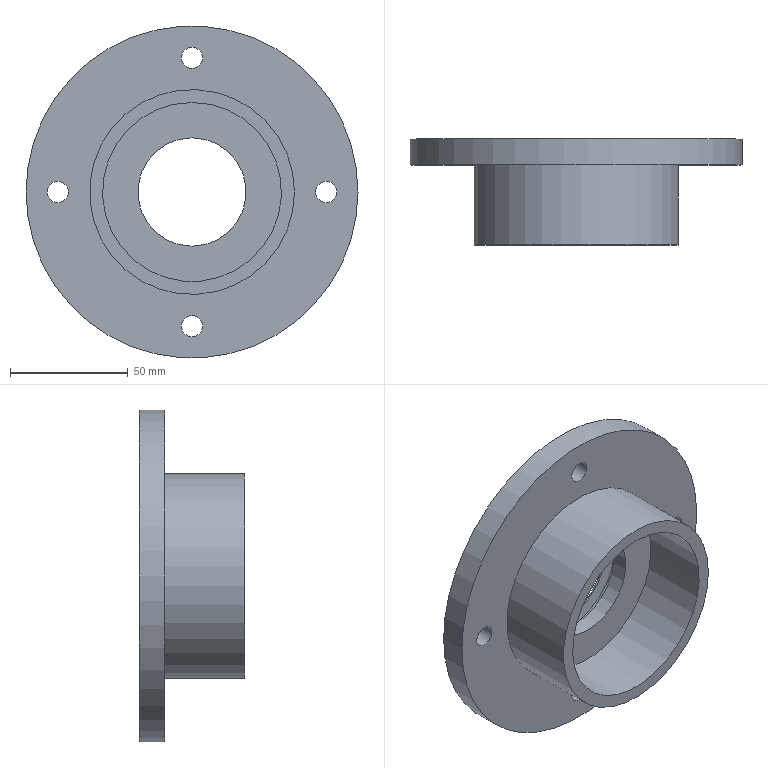Part | NX | features DATUM_CSYS 8, HOLE PACKAGE 7, SIMPLE HOLE 7, SKETCH 7, EXTRACT_DATUM_AXIS 4, EXTRACT_FACE 4, Instance Feature 3, EXTRUDE 2, Pattern Feature 1, SWP104 1 | 1 solid | 18 faces | box 141 x 45 x 141 mm | volume 198778 mm3 | cylinder 11 | plane 5 | cone 2 | commonest cylinder face diameters 9 x4 46 x2 56 x1 76 x1 81 x1 87 x1
STEP:
#1=CARTESIAN_POINT('',(0.,-16.,23.));
#2=VERTEX_POINT('',#1);
#3=CARTESIAN_POINT('',(0.,-16.,0.));
#4=DIRECTION('',(0.,1.,0.));
#5=DIRECTION('',(0.,0.,1.));
#6=AXIS2_PLACEMENT_3D('',#3,#4,#5);
#7=CIRCLE('',#6,23.);
#8=EDGE_CURVE('',#2,#2,#7,.F.);
#9=ORIENTED_EDGE('',*,*,#8,.T.);
#10=EDGE_LOOP('',(#9));
#11=FACE_BOUND('',#10,.T.);
#12=CARTESIAN_POINT('',(0.,-8.929,23.));
#13=VERTEX_POINT('',#12);
#14=CARTESIAN_POINT('',(0.,-8.929,0.));
#15=DIRECTION('',(0.,1.,0.));
#16=DIRECTION('',(0.,0.,1.));
#17=AXIS2_PLACEMENT_3D('',#14,#15,#16);
#18=CIRCLE('',#17,23.);
#19=EDGE_CURVE('',#13,#13,#18,.F.);
#20=ORIENTED_EDGE('',*,*,#19,.F.);
#21=EDGE_LOOP('',(#20));
#22=FACE_BOUND('',#21,.T.);
#23=CARTESIAN_POINT('',(0.,-45.,0.));
#24=DIRECTION('',(0.,1.,0.));
#25=DIRECTION('',(0.,0.,1.));
#26=AXIS2_PLACEMENT_3D('',#23,#24,#25);
#27=CYLINDRICAL_SURFACE('',#26,23.);
#28=ADVANCED_FACE('',(#11,#22),#27,.F.);
#29=CARTESIAN_POINT('',(0.,-3.,-23.));
#30=VERTEX_POINT('',#29);
#31=CARTESIAN_POINT('',(0.,-3.,0.));
#32=DIRECTION('',(0.,-1.,0.));
#33=DIRECTION('',(0.,0.,-1.));
#34=AXIS2_PLACEMENT_3D('',#31,#32,#33);
#35=CIRCLE('',#34,23.);
#36=EDGE_CURVE('',#30,#30,#35,.F.);
#37=ORIENTED_EDGE('',*,*,#36,.T.);
#38=EDGE_LOOP('',(#37));
#39=FACE_BOUND('',#38,.T.);
#40=CARTESIAN_POINT('',(0.,-3.702,-23.));
#41=VERTEX_POINT('',#40);
#42=CARTESIAN_POINT('',(0.,-3.702,0.));
#43=DIRECTION('',(0.,-1.,0.));
#44=DIRECTION('',(0.,0.,-1.));
#45=AXIS2_PLACEMENT_3D('',#42,#43,#44);
#46=CIRCLE('',#45,23.);
#47=EDGE_CURVE('',#41,#41,#46,.T.);
#48=ORIENTED_EDGE('',*,*,#47,.T.);
#49=EDGE_LOOP('',(#48));
#50=FACE_BOUND('',#49,.T.);
#51=CARTESIAN_POINT('',(0.,-45.,0.));
#52=DIRECTION('',(0.,1.,0.));
#53=DIRECTION('',(0.,0.,1.));
#54=AXIS2_PLACEMENT_3D('',#51,#52,#53);
#55=CYLINDRICAL_SURFACE('',#54,23.);
#56=ADVANCED_FACE('',(#39,#50),#55,.F.);
#57=CARTESIAN_POINT('',(70.5,-11.,0.));
#58=VERTEX_POINT('',#57);
#59=CARTESIAN_POINT('',(0.,-11.,0.));
#60=DIRECTION('',(0.,-1.,0.));
#61=DIRECTION('',(1.,0.,0.));
#62=AXIS2_PLACEMENT_3D('',#59,#60,#61);
#63=CIRCLE('',#62,70.5);
#64=EDGE_CURVE('',#58,#58,#63,.T.);
#65=ORIENTED_EDGE('',*,*,#64,.F.);
#66=EDGE_LOOP('',(#65));
#67=FACE_BOUND('',#66,.T.);
#68=CARTESIAN_POINT('',(70.5,0.,0.));
#69=VERTEX_POINT('',#68);
#70=CARTESIAN_POINT('',(0.,0.,0.));
#71=DIRECTION('',(0.,-1.,0.));
#72=DIRECTION('',(1.,0.,0.));
#73=AXIS2_PLACEMENT_3D('',#70,#71,#72);
#74=CIRCLE('',#73,70.5);
#75=EDGE_CURVE('',#69,#69,#74,.T.);
#76=ORIENTED_EDGE('',*,*,#75,.T.);
#77=EDGE_LOOP('',(#76));
#78=FACE_BOUND('',#77,.T.);
#79=CARTESIAN_POINT('',(0.,-11.,0.));
#80=DIRECTION('',(0.,1.,0.));
#81=DIRECTION('',(0.,0.,1.));
#82=AXIS2_PLACEMENT_3D('',#79,#80,#81);
#83=CYLINDRICAL_SURFACE('',#82,70.5);
#84=ADVANCED_FACE('',(#67,#78),#83,.T.);
#85=CARTESIAN_POINT('',(0.,-11.,-61.5));
#86=VERTEX_POINT('',#85);
#87=CARTESIAN_POINT('',(0.,-11.,-57.));
#88=DIRECTION('',(0.,-1.,0.));
#89=DIRECTION('',(0.,0.,-1.));
#90=AXIS2_PLACEMENT_3D('',#87,#88,#89);
#91=CIRCLE('',#90,4.5);
#92=EDGE_CURVE('',#86,#86,#91,.T.);
#93=ORIENTED_EDGE('',*,*,#92,.F.);
#94=EDGE_LOOP('',(#93));
#95=FACE_BOUND('',#94,.T.);
#96=CARTESIAN_POINT('',(57.,-11.,-4.5));
#97=VERTEX_POINT('',#96);
#98=CARTESIAN_POINT('',(57.,-11.,0.));
#99=DIRECTION('',(0.,-1.,0.));
#100=DIRECTION('',(0.,0.,-1.));
#101=AXIS2_PLACEMENT_3D('',#98,#99,#100);
#102=CIRCLE('',#101,4.5);
#103=EDGE_CURVE('',#97,#97,#102,.T.);
#104=ORIENTED_EDGE('',*,*,#103,.F.);
#105=EDGE_LOOP('',(#104));
#106=FACE_BOUND('',#105,.T.);
#107=CARTESIAN_POINT('',(0.,-11.,52.5));
#108=VERTEX_POINT('',#107);
#109=CARTESIAN_POINT('',(0.,-11.,57.));
#110=DIRECTION('',(0.,-1.,0.));
#111=DIRECTION('',(0.,0.,-1.));
#112=AXIS2_PLACEMENT_3D('',#109,#110,#111);
#113=CIRCLE('',#112,4.5);
#114=EDGE_CURVE('',#108,#108,#113,.T.);
#115=ORIENTED_EDGE('',*,*,#114,.F.);
#116=EDGE_LOOP('',(#115));
#117=FACE_BOUND('',#116,.T.);
#118=CARTESIAN_POINT('',(-57.,-11.,-4.5));
#119=VERTEX_POINT('',#118);
#120=CARTESIAN_POINT('',(-57.,-11.,0.));
#121=DIRECTION('',(0.,-1.,0.));
#122=DIRECTION('',(0.,0.,-1.));
#123=AXIS2_PLACEMENT_3D('',#120,#121,#122);
#124=CIRCLE('',#123,4.5);
#125=EDGE_CURVE('',#119,#119,#124,.T.);
#126=ORIENTED_EDGE('',*,*,#125,.F.);
#127=EDGE_LOOP('',(#126));
#128=FACE_BOUND('',#127,.T.);
#129=CARTESIAN_POINT('',(43.5,-11.,0.));
#130=VERTEX_POINT('',#129);
#131=CARTESIAN_POINT('',(0.,-11.,0.));
#132=DIRECTION('',(0.,-1.,0.));
#133=DIRECTION('',(1.,0.,0.));
#134=AXIS2_PLACEMENT_3D('',#131,#132,#133);
#135=CIRCLE('',#134,43.5);
#136=EDGE_CURVE('',#130,#130,#135,.T.);
#137=ORIENTED_EDGE('',*,*,#136,.F.);
#138=EDGE_LOOP('',(#137));
#139=FACE_BOUND('',#138,.T.);
#140=ORIENTED_EDGE('',*,*,#64,.T.);
#141=EDGE_LOOP('',(#140));
#142=FACE_BOUND('',#141,.T.);
#143=CARTESIAN_POINT('',(0.,-11.,0.));
#144=DIRECTION('',(0.,-1.,0.));
#145=DIRECTION('',(0.,0.,-1.));
#146=AXIS2_PLACEMENT_3D('',#143,#144,#145);
#147=PLANE('',#146);
#148=ADVANCED_FACE('',(#95,#106,#117,#128,#139,#142),#147,.T.);
#149=CARTESIAN_POINT('',(0.,0.,-61.5));
#150=VERTEX_POINT('',#149);
#151=CARTESIAN_POINT('',(0.,0.,-57.));
#152=DIRECTION('',(0.,-1.,0.));
#153=DIRECTION('',(0.,0.,-1.));
#154=AXIS2_PLACEMENT_3D('',#151,#152,#153);
#155=CIRCLE('',#154,4.5);
#156=EDGE_CURVE('',#150,#150,#155,.T.);
#157=ORIENTED_EDGE('',*,*,#156,.T.);
#158=EDGE_LOOP('',(#157));
#159=FACE_BOUND('',#158,.T.);
#160=CARTESIAN_POINT('',(57.,0.,-4.5));
#161=VERTEX_POINT('',#160);
#162=CARTESIAN_POINT('',(57.,0.,0.));
#163=DIRECTION('',(0.,-1.,0.));
#164=DIRECTION('',(0.,0.,-1.));
#165=AXIS2_PLACEMENT_3D('',#162,#163,#164);
#166=CIRCLE('',#165,4.5);
#167=EDGE_CURVE('',#161,#161,#166,.T.);
#168=ORIENTED_EDGE('',*,*,#167,.T.);
#169=EDGE_LOOP('',(#168));
#170=FACE_BOUND('',#169,.T.);
#171=CARTESIAN_POINT('',(0.,0.,52.5));
#172=VERTEX_POINT('',#171);
#173=CARTESIAN_POINT('',(0.,0.,57.));
#174=DIRECTION('',(0.,-1.,0.));
#175=DIRECTION('',(0.,0.,-1.));
#176=AXIS2_PLACEMENT_3D('',#173,#174,#175);
#177=CIRCLE('',#176,4.5);
#178=EDGE_CURVE('',#172,#172,#177,.T.);
#179=ORIENTED_EDGE('',*,*,#178,.T.);
#180=EDGE_LOOP('',(#179));
#181=FACE_BOUND('',#180,.T.);
#182=CARTESIAN_POINT('',(-57.,0.,-4.5));
#183=VERTEX_POINT('',#182);
#184=CARTESIAN_POINT('',(-57.,0.,0.));
#185=DIRECTION('',(0.,-1.,0.));
#186=DIRECTION('',(0.,0.,-1.));
#187=AXIS2_PLACEMENT_3D('',#184,#185,#186);
#188=CIRCLE('',#187,4.5);
#189=EDGE_CURVE('',#183,#183,#188,.T.);
#190=ORIENTED_EDGE('',*,*,#189,.T.);
#191=EDGE_LOOP('',(#190));
#192=FACE_BOUND('',#191,.T.);
#193=CARTESIAN_POINT('',(0.,0.,-40.5));
#194=VERTEX_POINT('',#193);
#195=CARTESIAN_POINT('',(0.,0.,0.));
#196=DIRECTION('',(0.,-1.,0.));
#197=DIRECTION('',(0.,0.,-1.));
#198=AXIS2_PLACEMENT_3D('',#195,#196,#197);
#199=CIRCLE('',#198,40.5);
#200=EDGE_CURVE('',#194,#194,#199,.T.);
#201=ORIENTED_EDGE('',*,*,#200,.T.);
#202=EDGE_LOOP('',(#201));
#203=FACE_BOUND('',#202,.T.);
#204=ORIENTED_EDGE('',*,*,#75,.F.);
#205=EDGE_LOOP('',(#204));
#206=FACE_BOUND('',#205,.T.);
#207=CARTESIAN_POINT('',(0.,0.,0.));
#208=DIRECTION('',(0.,-1.,0.));
#209=DIRECTION('',(0.,0.,-1.));
#210=AXIS2_PLACEMENT_3D('',#207,#208,#209);
#211=PLANE('',#210);
#212=ADVANCED_FACE('',(#159,#170,#181,#192,#203,#206),#211,.F.);
#213=CARTESIAN_POINT('',(43.5,-45.,0.));
#214=VERTEX_POINT('',#213);
#215=CARTESIAN_POINT('',(0.,-45.,0.));
#216=DIRECTION('',(0.,-1.,0.));
#217=DIRECTION('',(1.,0.,0.));
#218=AXIS2_PLACEMENT_3D('',#215,#216,#217);
#219=CIRCLE('',#218,43.5);
#220=EDGE_CURVE('',#214,#214,#219,.T.);
#221=ORIENTED_EDGE('',*,*,#220,.F.);
#222=EDGE_LOOP('',(#221));
#223=FACE_BOUND('',#222,.T.);
#224=ORIENTED_EDGE('',*,*,#136,.T.);
#225=EDGE_LOOP('',(#224));
#226=FACE_BOUND('',#225,.T.);
#227=CARTESIAN_POINT('',(0.,-45.,0.));
#228=DIRECTION('',(0.,1.,0.));
#229=DIRECTION('',(0.,0.,1.));
#230=AXIS2_PLACEMENT_3D('',#227,#228,#229);
#231=CYLINDRICAL_SURFACE('',#230,43.5);
#232=ADVANCED_FACE('',(#223,#226),#231,.T.);
#233=CARTESIAN_POINT('',(0.,-45.,38.));
#234=VERTEX_POINT('',#233);
#235=CARTESIAN_POINT('',(0.,-45.,0.));
#236=DIRECTION('',(0.,1.,0.));
#237=DIRECTION('',(0.,0.,1.));
#238=AXIS2_PLACEMENT_3D('',#235,#236,#237);
#239=CIRCLE('',#238,38.);
#240=EDGE_CURVE('',#234,#234,#239,.T.);
#241=ORIENTED_EDGE('',*,*,#240,.T.);
#242=EDGE_LOOP('',(#241));
#243=FACE_BOUND('',#242,.T.);
#244=ORIENTED_EDGE('',*,*,#220,.T.);
#245=EDGE_LOOP('',(#244));
#246=FACE_BOUND('',#245,.T.);
#247=CARTESIAN_POINT('',(0.,-45.,0.));
#248=DIRECTION('',(0.,-1.,0.));
#249=DIRECTION('',(0.,0.,-1.));
#250=AXIS2_PLACEMENT_3D('',#247,#248,#249);
#251=PLANE('',#250);
#252=ADVANCED_FACE('',(#243,#246),#251,.T.);
#253=CARTESIAN_POINT('',(0.,-16.,38.));
#254=VERTEX_POINT('',#253);
#255=CARTESIAN_POINT('',(0.,-16.,0.));
#256=DIRECTION('',(0.,1.,0.));
#257=DIRECTION('',(0.,0.,1.));
#258=AXIS2_PLACEMENT_3D('',#255,#256,#257);
#259=CIRCLE('',#258,38.);
#260=EDGE_CURVE('',#254,#254,#259,.F.);
#261=ORIENTED_EDGE('',*,*,#260,.T.);
#262=EDGE_LOOP('',(#261));
#263=FACE_BOUND('',#262,.T.);
#264=ORIENTED_EDGE('',*,*,#8,.F.);
#265=EDGE_LOOP('',(#264));
#266=FACE_BOUND('',#265,.T.);
#267=CARTESIAN_POINT('',(0.,-16.,0.));
#268=DIRECTION('',(0.,1.,0.));
#269=DIRECTION('',(0.,0.,1.));
#270=AXIS2_PLACEMENT_3D('',#267,#268,#269);
#271=PLANE('',#270);
#272=ADVANCED_FACE('',(#263,#266),#271,.F.);
#273=ORIENTED_EDGE('',*,*,#260,.F.);
#274=EDGE_LOOP('',(#273));
#275=FACE_BOUND('',#274,.T.);
#276=ORIENTED_EDGE('',*,*,#240,.F.);
#277=EDGE_LOOP('',(#276));
#278=FACE_BOUND('',#277,.T.);
#279=CARTESIAN_POINT('',(0.,-45.,0.));
#280=DIRECTION('',(0.,1.,0.));
#281=DIRECTION('',(0.,0.,1.));
#282=AXIS2_PLACEMENT_3D('',#279,#280,#281);
#283=CYLINDRICAL_SURFACE('',#282,38.);
#284=ADVANCED_FACE('',(#275,#278),#283,.F.);
#285=CARTESIAN_POINT('',(0.,-3.,-40.5));
#286=VERTEX_POINT('',#285);
#287=CARTESIAN_POINT('',(0.,-3.,0.));
#288=DIRECTION('',(0.,-1.,0.));
#289=DIRECTION('',(0.,0.,-1.));
#290=AXIS2_PLACEMENT_3D('',#287,#288,#289);
#291=CIRCLE('',#290,40.5);
#292=EDGE_CURVE('',#286,#286,#291,.F.);
#293=ORIENTED_EDGE('',*,*,#292,.T.);
#294=EDGE_LOOP('',(#293));
#295=FACE_BOUND('',#294,.T.);
#296=ORIENTED_EDGE('',*,*,#36,.F.);
#297=EDGE_LOOP('',(#296));
#298=FACE_BOUND('',#297,.T.);
#299=CARTESIAN_POINT('',(0.,-3.,0.));
#300=DIRECTION('',(0.,-1.,0.));
#301=DIRECTION('',(0.,0.,-1.));
#302=AXIS2_PLACEMENT_3D('',#299,#300,#301);
#303=PLANE('',#302);
#304=ADVANCED_FACE('',(#295,#298),#303,.F.);
#305=ORIENTED_EDGE('',*,*,#292,.F.);
#306=EDGE_LOOP('',(#305));
#307=FACE_BOUND('',#306,.T.);
#308=ORIENTED_EDGE('',*,*,#200,.F.);
#309=EDGE_LOOP('',(#308));
#310=FACE_BOUND('',#309,.T.);
#311=CARTESIAN_POINT('',(0.,0.,0.));
#312=DIRECTION('',(0.,-1.,0.));
#313=DIRECTION('',(0.,0.,-1.));
#314=AXIS2_PLACEMENT_3D('',#311,#312,#313);
#315=CYLINDRICAL_SURFACE('',#314,40.5);
#316=ADVANCED_FACE('',(#307,#310),#315,.F.);
#317=CARTESIAN_POINT('',(0.,-8.315,-28.));
#318=VERTEX_POINT('',#317);
#319=CARTESIAN_POINT('',(0.,-8.315,0.));
#320=DIRECTION('',(0.,-1.,0.));
#321=DIRECTION('',(0.,0.,-1.));
#322=AXIS2_PLACEMENT_3D('',#319,#320,#321);
#323=CIRCLE('',#322,28.);
#324=EDGE_CURVE('',#318,#318,#323,.F.);
#325=ORIENTED_EDGE('',*,*,#324,.T.);
#326=EDGE_LOOP('',(#325));
#327=FACE_BOUND('',#326,.T.);
#328=ORIENTED_EDGE('',*,*,#19,.T.);
#329=EDGE_LOOP('',(#328));
#330=FACE_BOUND('',#329,.T.);
#331=CARTESIAN_POINT('',(0.,-8.315,0.));
#332=DIRECTION('',(0.,1.,0.));
#333=DIRECTION('',(0.,0.,1.));
#334=AXIS2_PLACEMENT_3D('',#331,#332,#333);
#335=CONICAL_SURFACE('',#334,28.,1.449);
#336=ADVANCED_FACE('',(#327,#330),#335,.F.);
#337=CARTESIAN_POINT('',(0.,-4.315,-28.));
#338=VERTEX_POINT('',#337);
#339=CARTESIAN_POINT('',(0.,-4.315,0.));
#340=DIRECTION('',(0.,-1.,0.));
#341=DIRECTION('',(0.,0.,-1.));
#342=AXIS2_PLACEMENT_3D('',#339,#340,#341);
#343=CIRCLE('',#342,28.);
#344=EDGE_CURVE('',#338,#338,#343,.F.);
#345=ORIENTED_EDGE('',*,*,#344,.F.);
#346=EDGE_LOOP('',(#345));
#347=FACE_BOUND('',#346,.T.);
#348=ORIENTED_EDGE('',*,*,#47,.F.);
#349=EDGE_LOOP('',(#348));
#350=FACE_BOUND('',#349,.T.);
#351=CARTESIAN_POINT('',(0.,-3.456,0.));
#352=DIRECTION('',(0.,-1.,0.));
#353=DIRECTION('',(0.,0.,-1.));
#354=AXIS2_PLACEMENT_3D('',#351,#352,#353);
#355=CONICAL_SURFACE('',#354,21.,1.449);
#356=ADVANCED_FACE('',(#347,#350),#355,.F.);
#357=ORIENTED_EDGE('',*,*,#324,.F.);
#358=EDGE_LOOP('',(#357));
#359=FACE_BOUND('',#358,.T.);
#360=ORIENTED_EDGE('',*,*,#344,.T.);
#361=EDGE_LOOP('',(#360));
#362=FACE_BOUND('',#361,.T.);
#363=CARTESIAN_POINT('',(0.,0.,0.));
#364=DIRECTION('',(0.,-1.,0.));
#365=DIRECTION('',(0.,0.,-1.));
#366=AXIS2_PLACEMENT_3D('',#363,#364,#365);
#367=CYLINDRICAL_SURFACE('',#366,28.);
#368=ADVANCED_FACE('',(#359,#362),#367,.F.);
#369=ORIENTED_EDGE('',*,*,#125,.T.);
#370=EDGE_LOOP('',(#369));
#371=FACE_BOUND('',#370,.T.);
#372=ORIENTED_EDGE('',*,*,#189,.F.);
#373=EDGE_LOOP('',(#372));
#374=FACE_BOUND('',#373,.T.);
#375=CARTESIAN_POINT('',(-57.,0.,0.));
#376=DIRECTION('',(0.,-1.,0.));
#377=DIRECTION('',(0.,0.,-1.));
#378=AXIS2_PLACEMENT_3D('',#375,#376,#377);
#379=CYLINDRICAL_SURFACE('',#378,4.5);
#380=ADVANCED_FACE('',(#371,#374),#379,.F.);
#381=ORIENTED_EDGE('',*,*,#114,.T.);
#382=EDGE_LOOP('',(#381));
#383=FACE_BOUND('',#382,.T.);
#384=ORIENTED_EDGE('',*,*,#178,.F.);
#385=EDGE_LOOP('',(#384));
#386=FACE_BOUND('',#385,.T.);
#387=CARTESIAN_POINT('',(0.,0.,57.));
#388=DIRECTION('',(0.,-1.,0.));
#389=DIRECTION('',(0.,0.,-1.));
#390=AXIS2_PLACEMENT_3D('',#387,#388,#389);
#391=CYLINDRICAL_SURFACE('',#390,4.5);
#392=ADVANCED_FACE('',(#383,#386),#391,.F.);
#393=ORIENTED_EDGE('',*,*,#103,.T.);
#394=EDGE_LOOP('',(#393));
#395=FACE_BOUND('',#394,.T.);
#396=ORIENTED_EDGE('',*,*,#167,.F.);
#397=EDGE_LOOP('',(#396));
#398=FACE_BOUND('',#397,.T.);
#399=CARTESIAN_POINT('',(57.,0.,0.));
#400=DIRECTION('',(0.,-1.,0.));
#401=DIRECTION('',(0.,0.,-1.));
#402=AXIS2_PLACEMENT_3D('',#399,#400,#401);
#403=CYLINDRICAL_SURFACE('',#402,4.5);
#404=ADVANCED_FACE('',(#395,#398),#403,.F.);
#405=ORIENTED_EDGE('',*,*,#92,.T.);
#406=EDGE_LOOP('',(#405));
#407=FACE_BOUND('',#406,.T.);
#408=ORIENTED_EDGE('',*,*,#156,.F.);
#409=EDGE_LOOP('',(#408));
#410=FACE_BOUND('',#409,.T.);
#411=CARTESIAN_POINT('',(0.,0.,-57.));
#412=DIRECTION('',(0.,-1.,0.));
#413=DIRECTION('',(0.,0.,-1.));
#414=AXIS2_PLACEMENT_3D('',#411,#412,#413);
#415=CYLINDRICAL_SURFACE('',#414,4.5);
#416=ADVANCED_FACE('',(#407,#410),#415,.F.);
#417=CLOSED_SHELL('',(#28,#56,#84,#148,#212,#232,#252,#272,#284,#304,#316,#336,#356,#368,#380,#392,#404,#416));
#418=MANIFOLD_SOLID_BREP('',#417);
#419=(LENGTH_UNIT()NAMED_UNIT(*)SI_UNIT(.MILLI.,.METRE.));
#420=UNCERTAINTY_MEASURE_WITH_UNIT(LENGTH_MEASURE(0.00001),#419,'','');
#421=(NAMED_UNIT(*)PLANE_ANGLE_UNIT()SI_UNIT($,.RADIAN.));
#422=(NAMED_UNIT(*)SI_UNIT($,.STERADIAN.)SOLID_ANGLE_UNIT());
#423=(GEOMETRIC_REPRESENTATION_CONTEXT(3)GLOBAL_UNCERTAINTY_ASSIGNED_CONTEXT((#420))GLOBAL_UNIT_ASSIGNED_CONTEXT((#419,#421,#422))REPRESENTATION_CONTEXT('',''));
#424=ADVANCED_BREP_SHAPE_REPRESENTATION('',(#418),#423);